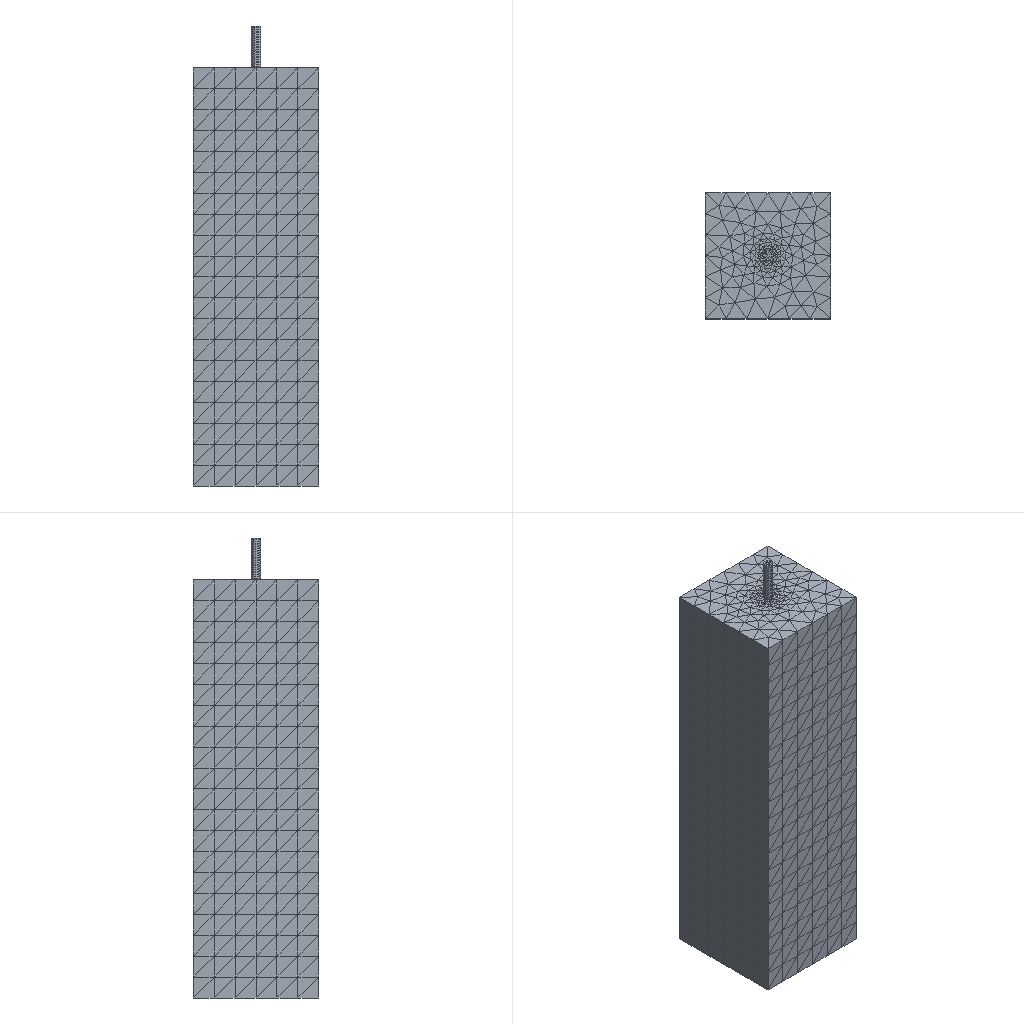Simulation study | abaqus
Set-up summary:
category,name,step,type,value,unit,region
solver,abaqus
solver,version,,,Abaqus/Explicit 2020
units,not stated in the deck,,not stated
analysis,deck,,transient,transient
load_step,Step-1,Step-1,transient
load_step,requested,,,1
mesh,nodes,,,21140
mesh,elements,,,101210
element_type,C3D4,,solid,101210
load,load commands in deck,,count,1
bc,support commands in deck,,count,3
material,MAO,,in results
material,SOIL,,in results
check,setup vs results,,match,"per instance, exact: element labels, types and connectivity; labels of the nodes the elements use; coordinates of those nodes at SINGLE_PRECISION in 2 of 2 instance(s)"
Abaqus input file, long lists of numbers shortened:
*Heading
** Job name: Job-3 Model name: Model-1-Copy-Copy
** Generated by: Abaqus/CAE 2020
*Preprint, echo=NO, model=NO, history=NO, contact=NO
**
** PARTS
**
*Part, name=merge-soil
*Node
      1,         150.,        -161.,         100.
      2,         150.,        -139.,         100.
** (11549 more lines like these left out)
*Element, type=C3D4
    1,  3425,  3426,  3427,  3428
    2,  3426,  3429,  3430,  3431
** (59732 more lines like these left out)
*Nset, nset=Set-4, generate
     1,  11551,      1
*Elset, elset=Set-4, generate
     1,  59734,      1
** Section: Section-1
*Solid Section, elset=Set-4, material=soil
,
*End Part
**
*Part, name=work
*Node
      1,   886.763,   1366.427,           5.
      2,   936.763,   1366.427,           5.
** (9587 more lines like these left out)
*Element, type=C3D4
   1, 5041, 5042, 5043, 1479
   2, 5041, 5042, 1479, 5044
** (41474 more lines like these left out)
*Nset, nset=Set-3, generate
    1,  9589,     1
*Elset, elset=Set-3, generate
     1,  41476,      1
** Section: Section-2
*Solid Section, elset=Set-3, material=mao
,
*End Part
**
**
** ASSEMBLY
**
*Assembly, name=Assembly
**
*Instance, name=work-1, part=work
        150.,  -1527.428,  -786.763
        150.,  -1527.428,  -786.763,         150., -1528.428,  -786.763, 90.
*End Instance
**
*Instance, name=merge-soil-1, part=merge-soil
*End Instance
**
*Node
      1,         150.,        -150.,        1100.
*Nset, nset=Set-7
 1,
*Nset, nset=Set-8, instance=merge-soil-1
   83,   84,   88,   89,  868,  869,  870,  871,  872,  946,  947,  948,  949,  950,  951,  952
  953,  954,  955,  956,  957,  958,  959,  960, 3080, 3081, 3082, 3083, 3084, 3085, 3086, 3087
** (2 more lines like these left out)
*Elset, elset=Set-8, instance=merge-soil-1
    27,   212,   546,   849,  1280,  5200,  5771,  5841,  5878,  5913,  5968,  6025, 13187, 13203, 22926, 22977
 23119, 23134, 23172, 23202, 23214, 25065, 25084, 25093, 25125, 25163, 25205, 25211, 25224, 25228, 25244, 25248
** (3 more lines like these left out)
*Nset, nset=Set-9, instance=merge-soil-1
   81,   82,   83,   84,   87,   88,   89,   90,  844,  845,  846,  847,  848,  849,  850,  851
  852,  853,  854,  855,  856,  857,  858,  859,  860,  861,  862,  863,  864,  865,  866,  867
** (17 more lines like these left out)
*Elset, elset=Set-9, instance=merge-soil-1
    30,   202,   218,   255,   258,   411,   426,   502,   686,   720,   752,   759,   847,   968,  1178,  1188
  1591,  1840,  2023,  2037,  2267,  2277,  2485,  2521,  2848,  2934,  2935,  2981,  3281,  3794,  4147,  4233
** (28 more lines like these left out)
*Nset, nset=Set-10, instance=merge-soil-1
   81,   82,   83,   84,   87,   88,   89,   90,  849,  850,  851,  852,  853,  854,  855,  856
  857,  858,  859,  860,  861,  862,  863,  864,  865,  866,  867,  873,  874,  875,  876,  877
** (17 more lines like these left out)
*Elset, elset=Set-10, instance=merge-soil-1
   533,   571,   768,  1469,  1624,  1671,  1711,  1899,  1906,  1948,  2270,  2504,  2787,  3057,  3059,  3220
  3593,  3799,  4011,  4339,  4666,  4721,  4969,  5109,  5164,  5190,  5261,  5308,  5313,  5331,  5460,  5479
** (28 more lines like these left out)
*Nset, nset=m_Set-6
 1,
*Elset, elset=_m_Surf-2_S1, internal, instance=work-1
  1405,  1567,  1612,  2145,  2241,  2452,  2467,  2501,  3164,  3190,  3293,  3299,  3343,  3513,  3847,  5128
  5130,  5157,  6045,  6722,  6811,  7113,  8618,  8630,  8702,  8894,  9035,  9051,  9118,  9163,  9418,  9978
** (86 more lines like these left out)
*Elset, elset=_m_Surf-2_S2, internal, instance=work-1
  1567,  1572,  1612,  1811,  1879,  1983,  1986,  2246,  2247,  2312,  2318,  2324,  2470,  2885,  2926,  3188
  3194,  3208,  3218,  3403,  3502,  3782,  3904,  4210,  4256,  4267,  4505,  4790,  5727,  8293,  8937,  9171
** (88 more lines like these left out)
*Elset, elset=_m_Surf-2_S3, internal, instance=work-1
    65,   108,   119,   210,   211,   360,   398,   430,   455,   459,   485,   487,   556,   578,   662,   735
   797,   798,   811,   828,   841,   854,   856,   858,   866,   887,   890,   894,   903,   911,   915,   919
** (418 more lines like these left out)
*Elset, elset=_m_Surf-2_S4, internal, instance=work-1
   184,   206,   246,  1757,  1884,  1888,  2138,  2239,  2326,  2882,  2885,  2973,  3055,  3164,  3534,  3877
  3916,  4040,  4054,  4291,  4308,  4334,  4359,  4379,  4386,  4394,  4531,  4551,  4790,  5023,  7290,  7643
** (25 more lines like these left out)
*Surface, type=ELEMENT, name=m_Surf-2
_m_Surf-2_S1, S1
_m_Surf-2_S2, S2
_m_Surf-2_S4, S4
_m_Surf-2_S3, S3
*Elset, elset=_s_Surf-1_S1, internal, instance=work-1
  6373, 30061
*Elset, elset=_s_Surf-1_S4, internal, instance=work-1
  6375, 11300, 15639, 39088
*Elset, elset=_s_Surf-1_S3, internal, instance=work-1
  9925,  9955, 10341, 11160, 11198, 11200, 11214, 11221, 11225, 11230, 11243, 11248, 11249, 11267, 11278, 11292
 11297, 11298, 11304, 11306, 11320, 11353, 11366, 11367, 11684, 11693, 11698, 11700, 11713, 11714, 11740, 11760
** (1 more lines like these left out)
*Elset, elset=_s_Surf-1_S2, internal, instance=work-1
 11323,
*Surface, type=ELEMENT, name=s_Surf-1
_s_Surf-1_S1, S1
_s_Surf-1_S4, S4
_s_Surf-1_S2, S2
_s_Surf-1_S3, S3
*Elset, elset=_s_Surf-4_S1, internal, instance=merge-soil-1
  1542,  3389,  5092,  5223,  5302,  5311,  5333,  5344,  5394,  5506,  5626,  5870,  5983,  6120,  6129,  6658
  6813,  6849,  6883,  6895,  6905,  6907,  6928,  6937,  6945,  7015,  7027,  7034,  7083,  7090,  7128,  7163
** (38 more lines like these left out)
*Elset, elset=_s_Surf-4_S3, internal, instance=merge-soil-1
   215,   284,   401,   677,   840,   945,   950,  1008,  1062,  1542,  1674,  1709,  1710,  1778,  2128,  2428
  2514,  2712,  2837,  2920,  2969,  3157,  3198,  3214,  3271,  3390,  3578,  3648,  3798,  4336,  4430,  4546
** (243 more lines like these left out)
*Elset, elset=_s_Surf-4_S4, internal, instance=merge-soil-1
  1523,  3656,  5293,  5453,  5511,  5569,  5628,  5650,  5673,  5677,  5773,  5778,  5983,  5998,  6067,  6094
  6125,  6141,  6190,  6353,  6430,  6437,  6448,  6975,  6978,  7053,  7090,  7132,  7297,  7452,  7475,  7497
** (22 more lines like these left out)
*Elset, elset=_s_Surf-4_S2, internal, instance=merge-soil-1
   133,   503,  1774,  2026,  2562,  5086,  5094,  5155,  5178,  5518,  5624,  5628,  5677,  5941,  6049,  6231
  6258,  6307,  6353,  6414,  6511,  6557,  6591,  6595,  6600,  6751,  6753,  6769,  6778,  6785,  6792,  6802
** (36 more lines like these left out)
*Surface, type=ELEMENT, name=s_Surf-4
_s_Surf-4_S1, S1
_s_Surf-4_S3, S3
_s_Surf-4_S4, S4
_s_Surf-4_S2, S2
** Constraint: Constraint-1
*Coupling, constraint name=Constraint-1, ref node=m_Set-6, surface=s_Surf-1
*Kinematic
*End Assembly
*Amplitude, name=Amp-1
             0.,              0.,             0.1,              1.
**
** MATERIALS
**
*Material, name=mao
*Density
 7.8e-09,
*Elastic
140000., 0.32
*Plastic
348.,0.
*Material, name=soil
*Density
 2.7e-09,
*Elastic
5100., 0.25
*Mohr Coulomb
32., 0.1
*Mohr Coulomb Hardening
 4.6,0.
**
** INTERACTION PROPERTIES
**
*Surface Interaction, name=IntProp-1
*Friction
 0.2,
*Surface Behavior, pressure-overclosure=HARD
**
** BOUNDARY CONDITIONS
**
** Name: BC-1 Type: 对称/反对称/完全固定
*Boundary
Set-8, ENCASTRE
** Name: BC-2 Type: 位移/转角
*Boundary
Set-10, 2, 2
** Name: BC-3 Type: 位移/转角
*Boundary
Set-9, 1, 1
**
** INTERACTIONS
**
** Interaction: Int-2
*Contact, op=NEW
*Contact Inclusions, ALL EXTERIOR
*Contact Property Assignment
 ,  , IntProp-1
** ----------------------------------------------------------------
**
** STEP: Step-1
**
*Step, name=Step-1, nlgeom=YES
*Dynamic, Explicit
, 0.1
*Bulk Viscosity
0.06, 1.2
** Mass Scaling: Semi-Automatic
**               Whole Model
*Fixed Mass Scaling, factor=500.
**
** LOADS
**
** Name: Load-1   Type: Concentrated force
*Cload, amplitude=Amp-1
Set-7, 3, 100000.
**
** OUTPUT REQUESTS
**
*Restart, write, number interval=1, time marks=NO
**
** FIELD OUTPUT: F-Output-1
**
*Output, field, number interval=50
*Node Output
CF, RF, RM, RT, U, V
*Element Output, directions=YES
E, LE, MISES, MISESMAX, MISESONLY, PE, PEEQ, PEMAG, S, SF, SSAVG
*Contact Output
CDISP, CFORCE, CSTRESS
**
** HISTORY OUTPUT: H-Output-1
**
*Output, history, time interval=5e-05
*Node Output, nset=Set-7
U3, V3
*End Step
Results summary:
result,step,Step-1,completed,increments=148780 time=0.1/0.1
result,analysis,,,transient
result,last_loadstep,,,1
result,primary field,,,U
result,reaction total,,FX,24.715,model units
result,reaction total,,FY,-212.487,model units
result,reaction total,,FZ,-105970.707,model units